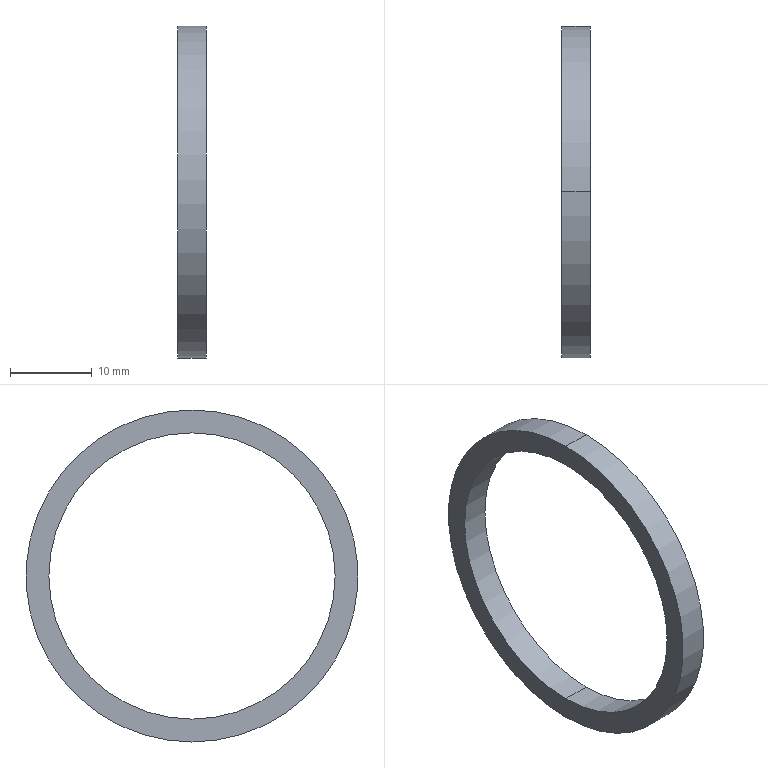Part | SolidWorks | features Extrusion 1 | 1 solid | 6 faces | box 3.5 x 40.6 x 40.6 mm | volume 1164 mm3 | cylinder 4 | plane 2 | commonest cylinder face diameters 35 x2 40.6 x2
STEP:
#1=CARTESIAN_POINT('',(3.5,0.,17.5));
#2=VERTEX_POINT('',#1);
#3=CARTESIAN_POINT('',(3.5,0.,-17.5));
#4=VERTEX_POINT('',#3);
#5=CARTESIAN_POINT('',(3.5,0.,0.));
#6=DIRECTION('',(1.,0.,0.));
#7=DIRECTION('',(0.,0.,-1.));
#8=AXIS2_PLACEMENT_3D('',#5,#6,#7);
#9=CIRCLE('',#8,17.5);
#10=EDGE_CURVE('',#2,#4,#9,.T.);
#11=ORIENTED_EDGE('',*,*,#10,.T.);
#12=CARTESIAN_POINT('',(0.,0.,-17.5));
#13=VERTEX_POINT('',#12);
#14=CARTESIAN_POINT('',(3.5,0.,-17.5));
#15=DIRECTION('',(-1.,0.,0.));
#16=VECTOR('',#15,1000.);
#17=LINE('',#14,#16);
#18=EDGE_CURVE('',#4,#13,#17,.T.);
#19=ORIENTED_EDGE('',*,*,#18,.T.);
#20=CARTESIAN_POINT('',(0.,0.,17.5));
#21=VERTEX_POINT('',#20);
#22=CARTESIAN_POINT('',(0.,0.,0.));
#23=DIRECTION('',(1.,0.,0.));
#24=DIRECTION('',(0.,0.,-1.));
#25=AXIS2_PLACEMENT_3D('',#22,#23,#24);
#26=CIRCLE('',#25,17.5);
#27=EDGE_CURVE('',#21,#13,#26,.T.);
#28=ORIENTED_EDGE('',*,*,#27,.F.);
#29=CARTESIAN_POINT('',(3.5,0.,17.5));
#30=DIRECTION('',(-1.,0.,0.));
#31=VECTOR('',#30,1000.);
#32=LINE('',#29,#31);
#33=EDGE_CURVE('',#2,#21,#32,.T.);
#34=ORIENTED_EDGE('',*,*,#33,.F.);
#35=EDGE_LOOP('',(#11,#19,#28,#34));
#36=FACE_OUTER_BOUND('',#35,.T.);
#37=CARTESIAN_POINT('',(3.5,0.,0.));
#38=DIRECTION('',(-1.,0.,0.));
#39=DIRECTION('',(0.,0.,1.));
#40=AXIS2_PLACEMENT_3D('',#37,#38,#39);
#41=CYLINDRICAL_SURFACE('',#40,17.5);
#42=ADVANCED_FACE('',(#36),#41,.F.);
#43=CARTESIAN_POINT('',(3.5,0.,-20.3));
#44=VERTEX_POINT('',#43);
#45=CARTESIAN_POINT('',(3.5,0.,20.3));
#46=VERTEX_POINT('',#45);
#47=CARTESIAN_POINT('',(3.5,0.,0.));
#48=DIRECTION('',(1.,0.,0.));
#49=DIRECTION('',(0.,0.,-1.));
#50=AXIS2_PLACEMENT_3D('',#47,#48,#49);
#51=CIRCLE('',#50,20.3);
#52=EDGE_CURVE('',#44,#46,#51,.T.);
#53=ORIENTED_EDGE('',*,*,#52,.F.);
#54=CARTESIAN_POINT('',(0.,0.,-20.3));
#55=VERTEX_POINT('',#54);
#56=CARTESIAN_POINT('',(3.5,0.,-20.3));
#57=DIRECTION('',(-1.,0.,0.));
#58=VECTOR('',#57,1000.);
#59=LINE('',#56,#58);
#60=EDGE_CURVE('',#44,#55,#59,.T.);
#61=ORIENTED_EDGE('',*,*,#60,.T.);
#62=CARTESIAN_POINT('',(0.,0.,20.3));
#63=VERTEX_POINT('',#62);
#64=CARTESIAN_POINT('',(0.,0.,0.));
#65=DIRECTION('',(1.,0.,0.));
#66=DIRECTION('',(0.,0.,-1.));
#67=AXIS2_PLACEMENT_3D('',#64,#65,#66);
#68=CIRCLE('',#67,20.3);
#69=EDGE_CURVE('',#55,#63,#68,.T.);
#70=ORIENTED_EDGE('',*,*,#69,.T.);
#71=CARTESIAN_POINT('',(3.5,0.,20.3));
#72=DIRECTION('',(-1.,0.,0.));
#73=VECTOR('',#72,1000.);
#74=LINE('',#71,#73);
#75=EDGE_CURVE('',#46,#63,#74,.T.);
#76=ORIENTED_EDGE('',*,*,#75,.F.);
#77=EDGE_LOOP('',(#53,#61,#70,#76));
#78=FACE_OUTER_BOUND('',#77,.T.);
#79=CARTESIAN_POINT('',(3.5,0.,0.));
#80=DIRECTION('',(-1.,0.,0.));
#81=DIRECTION('',(0.,0.,1.));
#82=AXIS2_PLACEMENT_3D('',#79,#80,#81);
#83=CYLINDRICAL_SURFACE('',#82,20.3);
#84=ADVANCED_FACE('',(#78),#83,.T.);
#85=CARTESIAN_POINT('',(3.5,0.,0.));
#86=DIRECTION('',(1.,0.,0.));
#87=DIRECTION('',(0.,0.,-1.));
#88=AXIS2_PLACEMENT_3D('',#85,#86,#87);
#89=CIRCLE('',#88,20.3);
#90=EDGE_CURVE('',#46,#44,#89,.T.);
#91=ORIENTED_EDGE('',*,*,#90,.T.);
#92=ORIENTED_EDGE('',*,*,#52,.T.);
#93=EDGE_LOOP('',(#91,#92));
#94=FACE_OUTER_BOUND('',#93,.T.);
#95=ORIENTED_EDGE('',*,*,#10,.F.);
#96=CARTESIAN_POINT('',(3.5,0.,0.));
#97=DIRECTION('',(1.,0.,0.));
#98=DIRECTION('',(0.,0.,-1.));
#99=AXIS2_PLACEMENT_3D('',#96,#97,#98);
#100=CIRCLE('',#99,17.5);
#101=EDGE_CURVE('',#4,#2,#100,.T.);
#102=ORIENTED_EDGE('',*,*,#101,.F.);
#103=EDGE_LOOP('',(#95,#102));
#104=FACE_BOUND('',#103,.T.);
#105=CARTESIAN_POINT('',(3.5,0.,0.));
#106=DIRECTION('',(1.,0.,0.));
#107=DIRECTION('',(0.,0.,-1.));
#108=AXIS2_PLACEMENT_3D('',#105,#106,#107);
#109=PLANE('',#108);
#110=ADVANCED_FACE('',(#94,#104),#109,.T.);
#111=CARTESIAN_POINT('',(0.,0.,0.));
#112=DIRECTION('',(1.,0.,0.));
#113=DIRECTION('',(0.,0.,-1.));
#114=AXIS2_PLACEMENT_3D('',#111,#112,#113);
#115=CIRCLE('',#114,20.3);
#116=EDGE_CURVE('',#63,#55,#115,.T.);
#117=ORIENTED_EDGE('',*,*,#116,.F.);
#118=ORIENTED_EDGE('',*,*,#69,.F.);
#119=EDGE_LOOP('',(#117,#118));
#120=FACE_OUTER_BOUND('',#119,.T.);
#121=ORIENTED_EDGE('',*,*,#27,.T.);
#122=CARTESIAN_POINT('',(0.,0.,0.));
#123=DIRECTION('',(1.,0.,0.));
#124=DIRECTION('',(0.,0.,-1.));
#125=AXIS2_PLACEMENT_3D('',#122,#123,#124);
#126=CIRCLE('',#125,17.5);
#127=EDGE_CURVE('',#13,#21,#126,.T.);
#128=ORIENTED_EDGE('',*,*,#127,.T.);
#129=EDGE_LOOP('',(#121,#128));
#130=FACE_BOUND('',#129,.T.);
#131=CARTESIAN_POINT('',(0.,0.,0.));
#132=DIRECTION('',(1.,0.,0.));
#133=DIRECTION('',(0.,0.,-1.));
#134=AXIS2_PLACEMENT_3D('',#131,#132,#133);
#135=PLANE('',#134);
#136=ADVANCED_FACE('',(#120,#130),#135,.F.);
#137=ORIENTED_EDGE('',*,*,#60,.F.);
#138=ORIENTED_EDGE('',*,*,#90,.F.);
#139=ORIENTED_EDGE('',*,*,#75,.T.);
#140=ORIENTED_EDGE('',*,*,#116,.T.);
#141=EDGE_LOOP('',(#137,#138,#139,#140));
#142=FACE_OUTER_BOUND('',#141,.T.);
#143=CARTESIAN_POINT('',(3.5,0.,0.));
#144=DIRECTION('',(-1.,0.,0.));
#145=DIRECTION('',(0.,0.,1.));
#146=AXIS2_PLACEMENT_3D('',#143,#144,#145);
#147=CYLINDRICAL_SURFACE('',#146,20.3);
#148=ADVANCED_FACE('',(#142),#147,.T.);
#149=ORIENTED_EDGE('',*,*,#18,.F.);
#150=ORIENTED_EDGE('',*,*,#101,.T.);
#151=ORIENTED_EDGE('',*,*,#33,.T.);
#152=ORIENTED_EDGE('',*,*,#127,.F.);
#153=EDGE_LOOP('',(#149,#150,#151,#152));
#154=FACE_OUTER_BOUND('',#153,.T.);
#155=CARTESIAN_POINT('',(3.5,0.,0.));
#156=DIRECTION('',(-1.,0.,0.));
#157=DIRECTION('',(0.,0.,1.));
#158=AXIS2_PLACEMENT_3D('',#155,#156,#157);
#159=CYLINDRICAL_SURFACE('',#158,17.5);
#160=ADVANCED_FACE('',(#154),#159,.F.);
#161=CLOSED_SHELL('',(#42,#84,#110,#136,#148,#160));
#162=MANIFOLD_SOLID_BREP('',#161);
#163=CARTESIAN_POINT('',(0.,0.,0.));
#164=DIRECTION('',(0.,0.,1.));
#165=DIRECTION('',(1.,0.,0.));
#166=AXIS2_PLACEMENT_3D('',#163,#164,#165);
#167=(LENGTH_UNIT()NAMED_UNIT(*)SI_UNIT(.MILLI.,.METRE.));
#168=UNCERTAINTY_MEASURE_WITH_UNIT(LENGTH_MEASURE(0.00001),#167,'','');
#169=(NAMED_UNIT(*)PLANE_ANGLE_UNIT()SI_UNIT($,.RADIAN.));
#170=(NAMED_UNIT(*)SI_UNIT($,.STERADIAN.)SOLID_ANGLE_UNIT());
#171=(GEOMETRIC_REPRESENTATION_CONTEXT(3)GLOBAL_UNCERTAINTY_ASSIGNED_CONTEXT((#168))GLOBAL_UNIT_ASSIGNED_CONTEXT((#167,#169,#170))REPRESENTATION_CONTEXT('',''));
#172=ADVANCED_BREP_SHAPE_REPRESENTATION('',(#162,#166),#171);